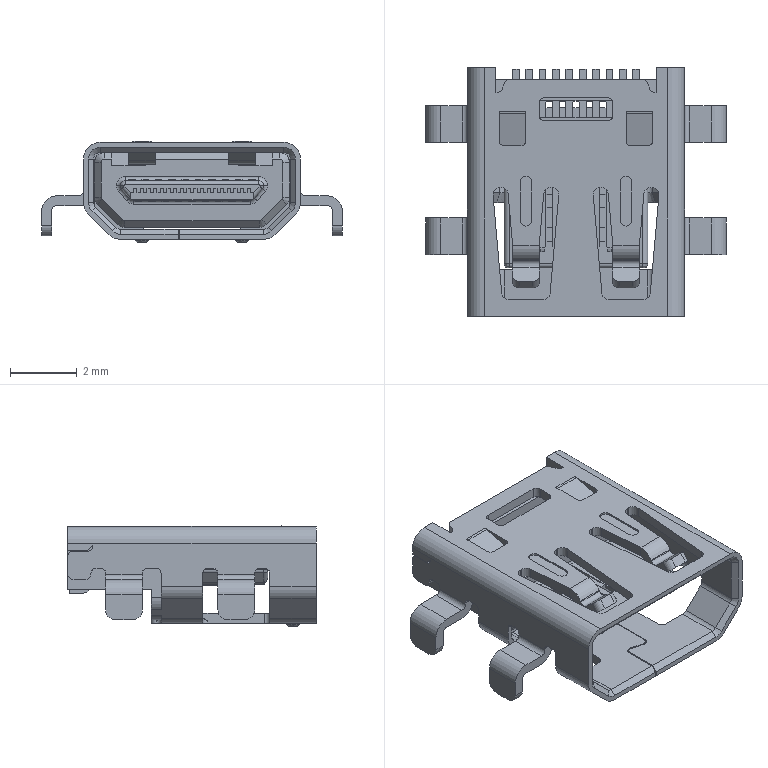Part | Creo | 1 solid | 886 faces | box 9 x 7.45 x 3.03 mm | volume 57.708 mm3 | plane 650 | cylinder 196 | cone 20 | torus 10 | spline 10 | commonest cylinder face diameters 0.3 x58 0.4 x32 0.48 x28 0.6 x16 1 x16 0.54 x10